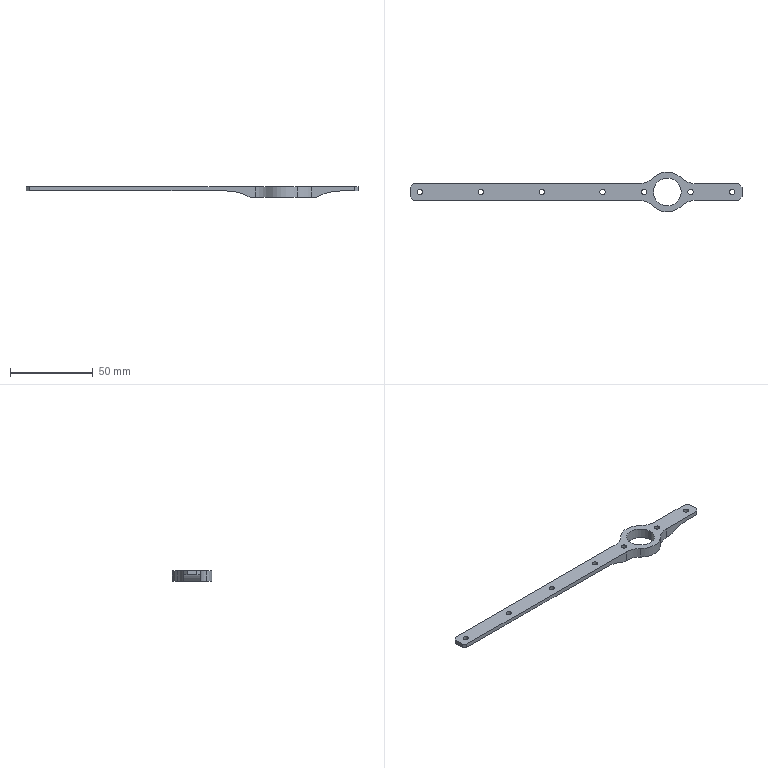Part | SolidWorks | features BaseBody 1 | 1 solid | 38 faces | box 200 x 24 x 6.35 mm | volume 6855 mm3 | cylinder 24 | plane 14 | commonest cylinder face diameters 3.2 x14 24 x6 16.667 x2 57.936 x2
STEP:
#1=CARTESIAN_POINT('',(46.666,0.,6.35));
#2=VERTEX_POINT('',#1);
#3=CARTESIAN_POINT('',(63.334,0.,6.35));
#4=VERTEX_POINT('',#3);
#5=CARTESIAN_POINT('',(55.,0.,6.35));
#6=DIRECTION('',(0.,0.,1.));
#7=DIRECTION('',(-1.,0.,0.));
#8=AXIS2_PLACEMENT_3D('',#5,#6,#7);
#9=CIRCLE('',#8,8.334);
#10=EDGE_CURVE('',#2,#4,#9,.T.);
#11=ORIENTED_EDGE('',*,*,#10,.T.);
#12=CARTESIAN_POINT('',(63.334,0.,0.));
#13=VERTEX_POINT('',#12);
#14=CARTESIAN_POINT('',(63.334,0.,6.35));
#15=DIRECTION('',(0.,0.,-1.));
#16=VECTOR('',#15,1000.);
#17=LINE('',#14,#16);
#18=EDGE_CURVE('',#4,#13,#17,.T.);
#19=ORIENTED_EDGE('',*,*,#18,.T.);
#20=CARTESIAN_POINT('',(46.666,0.,0.));
#21=VERTEX_POINT('',#20);
#22=CARTESIAN_POINT('',(55.,0.,0.));
#23=DIRECTION('',(0.,0.,-1.));
#24=DIRECTION('',(-1.,0.,0.));
#25=AXIS2_PLACEMENT_3D('',#22,#23,#24);
#26=CIRCLE('',#25,8.334);
#27=EDGE_CURVE('',#13,#21,#26,.T.);
#28=ORIENTED_EDGE('',*,*,#27,.T.);
#29=CARTESIAN_POINT('',(46.666,0.,6.35));
#30=DIRECTION('',(0.,0.,-1.));
#31=VECTOR('',#30,1000.);
#32=LINE('',#29,#31);
#33=EDGE_CURVE('',#2,#21,#32,.T.);
#34=ORIENTED_EDGE('',*,*,#33,.F.);
#35=EDGE_LOOP('',(#11,#19,#28,#34));
#36=FACE_OUTER_BOUND('',#35,.T.);
#37=CARTESIAN_POINT('',(55.,0.,6.35));
#38=DIRECTION('',(0.,0.,-1.));
#39=DIRECTION('',(-1.,0.,0.));
#40=AXIS2_PLACEMENT_3D('',#37,#38,#39);
#41=CYLINDRICAL_SURFACE('',#40,8.334);
#42=ADVANCED_FACE('',(#36),#41,.F.);
#43=CARTESIAN_POINT('',(67.4,0.,6.35));
#44=VERTEX_POINT('',#43);
#45=CARTESIAN_POINT('',(70.6,0.,6.35));
#46=VERTEX_POINT('',#45);
#47=CARTESIAN_POINT('',(69.,0.,6.35));
#48=DIRECTION('',(0.,0.,1.));
#49=DIRECTION('',(-1.,0.,0.));
#50=AXIS2_PLACEMENT_3D('',#47,#48,#49);
#51=CIRCLE('',#50,1.6);
#52=EDGE_CURVE('',#44,#46,#51,.T.);
#53=ORIENTED_EDGE('',*,*,#52,.T.);
#54=CARTESIAN_POINT('',(70.6,0.,0.));
#55=VERTEX_POINT('',#54);
#56=CARTESIAN_POINT('',(70.6,0.,6.35));
#57=DIRECTION('',(0.,0.,-1.));
#58=VECTOR('',#57,1000.);
#59=LINE('',#56,#58);
#60=EDGE_CURVE('',#46,#55,#59,.T.);
#61=ORIENTED_EDGE('',*,*,#60,.T.);
#62=CARTESIAN_POINT('',(67.4,0.,0.));
#63=VERTEX_POINT('',#62);
#64=CARTESIAN_POINT('',(69.,0.,0.));
#65=DIRECTION('',(0.,0.,1.));
#66=DIRECTION('',(-1.,0.,0.));
#67=AXIS2_PLACEMENT_3D('',#64,#65,#66);
#68=CIRCLE('',#67,1.6);
#69=EDGE_CURVE('',#63,#55,#68,.T.);
#70=ORIENTED_EDGE('',*,*,#69,.F.);
#71=CARTESIAN_POINT('',(67.4,0.,6.35));
#72=DIRECTION('',(0.,0.,-1.));
#73=VECTOR('',#72,1000.);
#74=LINE('',#71,#73);
#75=EDGE_CURVE('',#44,#63,#74,.T.);
#76=ORIENTED_EDGE('',*,*,#75,.F.);
#77=EDGE_LOOP('',(#53,#61,#70,#76));
#78=FACE_OUTER_BOUND('',#77,.T.);
#79=CARTESIAN_POINT('',(69.,0.,6.35));
#80=DIRECTION('',(0.,0.,-1.));
#81=DIRECTION('',(-1.,0.,0.));
#82=AXIS2_PLACEMENT_3D('',#79,#80,#81);
#83=CYLINDRICAL_SURFACE('',#82,1.6);
#84=ADVANCED_FACE('',(#78),#83,.F.);
#85=CARTESIAN_POINT('',(39.4,0.,6.35));
#86=VERTEX_POINT('',#85);
#87=CARTESIAN_POINT('',(42.6,0.,6.35));
#88=VERTEX_POINT('',#87);
#89=CARTESIAN_POINT('',(41.,0.,6.35));
#90=DIRECTION('',(0.,0.,1.));
#91=DIRECTION('',(-1.,0.,0.));
#92=AXIS2_PLACEMENT_3D('',#89,#90,#91);
#93=CIRCLE('',#92,1.6);
#94=EDGE_CURVE('',#86,#88,#93,.T.);
#95=ORIENTED_EDGE('',*,*,#94,.T.);
#96=CARTESIAN_POINT('',(42.6,0.,0.));
#97=VERTEX_POINT('',#96);
#98=CARTESIAN_POINT('',(42.6,0.,6.35));
#99=DIRECTION('',(0.,0.,-1.));
#100=VECTOR('',#99,1000.);
#101=LINE('',#98,#100);
#102=EDGE_CURVE('',#88,#97,#101,.T.);
#103=ORIENTED_EDGE('',*,*,#102,.T.);
#104=CARTESIAN_POINT('',(39.4,0.,0.));
#105=VERTEX_POINT('',#104);
#106=CARTESIAN_POINT('',(41.,0.,0.));
#107=DIRECTION('',(0.,0.,1.));
#108=DIRECTION('',(-1.,0.,0.));
#109=AXIS2_PLACEMENT_3D('',#106,#107,#108);
#110=CIRCLE('',#109,1.6);
#111=EDGE_CURVE('',#105,#97,#110,.T.);
#112=ORIENTED_EDGE('',*,*,#111,.F.);
#113=CARTESIAN_POINT('',(39.4,0.,6.35));
#114=DIRECTION('',(0.,0.,-1.));
#115=VECTOR('',#114,1000.);
#116=LINE('',#113,#115);
#117=EDGE_CURVE('',#86,#105,#116,.T.);
#118=ORIENTED_EDGE('',*,*,#117,.F.);
#119=EDGE_LOOP('',(#95,#103,#112,#118));
#120=FACE_OUTER_BOUND('',#119,.T.);
#121=CARTESIAN_POINT('',(41.,0.,6.35));
#122=DIRECTION('',(0.,0.,-1.));
#123=DIRECTION('',(-1.,0.,0.));
#124=AXIS2_PLACEMENT_3D('',#121,#122,#123);
#125=CYLINDRICAL_SURFACE('',#124,1.6);
#126=ADVANCED_FACE('',(#120),#125,.F.);
#127=CARTESIAN_POINT('',(-58.9,0.,6.35));
#128=VERTEX_POINT('',#127);
#129=CARTESIAN_POINT('',(-55.7,0.,6.35));
#130=VERTEX_POINT('',#129);
#131=CARTESIAN_POINT('',(-57.3,0.,6.35));
#132=DIRECTION('',(0.,0.,1.));
#133=DIRECTION('',(-1.,0.,0.));
#134=AXIS2_PLACEMENT_3D('',#131,#132,#133);
#135=CIRCLE('',#134,1.6);
#136=EDGE_CURVE('',#128,#130,#135,.T.);
#137=ORIENTED_EDGE('',*,*,#136,.T.);
#138=CARTESIAN_POINT('',(-55.7,0.,3.81));
#139=VERTEX_POINT('',#138);
#140=CARTESIAN_POINT('',(-55.7,0.,6.35));
#141=DIRECTION('',(0.,0.,-1.));
#142=VECTOR('',#141,1000.);
#143=LINE('',#140,#142);
#144=EDGE_CURVE('',#130,#139,#143,.T.);
#145=ORIENTED_EDGE('',*,*,#144,.T.);
#146=CARTESIAN_POINT('',(-58.9,0.,3.81));
#147=VERTEX_POINT('',#146);
#148=CARTESIAN_POINT('',(-57.3,0.,3.81));
#149=DIRECTION('',(0.,0.,-1.));
#150=DIRECTION('',(-1.,0.,0.));
#151=AXIS2_PLACEMENT_3D('',#148,#149,#150);
#152=CIRCLE('',#151,1.6);
#153=EDGE_CURVE('',#139,#147,#152,.T.);
#154=ORIENTED_EDGE('',*,*,#153,.T.);
#155=CARTESIAN_POINT('',(-58.9,0.,6.35));
#156=DIRECTION('',(0.,0.,-1.));
#157=VECTOR('',#156,1000.);
#158=LINE('',#155,#157);
#159=EDGE_CURVE('',#128,#147,#158,.T.);
#160=ORIENTED_EDGE('',*,*,#159,.F.);
#161=EDGE_LOOP('',(#137,#145,#154,#160));
#162=FACE_OUTER_BOUND('',#161,.T.);
#163=CARTESIAN_POINT('',(-57.3,0.,6.35));
#164=DIRECTION('',(0.,0.,-1.));
#165=DIRECTION('',(-1.,0.,0.));
#166=AXIS2_PLACEMENT_3D('',#163,#164,#165);
#167=CYLINDRICAL_SURFACE('',#166,1.6);
#168=ADVANCED_FACE('',(#162),#167,.F.);
#169=CARTESIAN_POINT('',(-22.25,0.,6.35));
#170=VERTEX_POINT('',#169);
#171=CARTESIAN_POINT('',(-19.05,0.,6.35));
#172=VERTEX_POINT('',#171);
#173=CARTESIAN_POINT('',(-20.65,0.,6.35));
#174=DIRECTION('',(0.,0.,1.));
#175=DIRECTION('',(-1.,0.,0.));
#176=AXIS2_PLACEMENT_3D('',#173,#174,#175);
#177=CIRCLE('',#176,1.6);
#178=EDGE_CURVE('',#170,#172,#177,.T.);
#179=ORIENTED_EDGE('',*,*,#178,.T.);
#180=CARTESIAN_POINT('',(-19.05,0.,3.81));
#181=VERTEX_POINT('',#180);
#182=CARTESIAN_POINT('',(-19.05,0.,6.35));
#183=DIRECTION('',(0.,0.,-1.));
#184=VECTOR('',#183,1000.);
#185=LINE('',#182,#184);
#186=EDGE_CURVE('',#172,#181,#185,.T.);
#187=ORIENTED_EDGE('',*,*,#186,.T.);
#188=CARTESIAN_POINT('',(-22.25,0.,3.81));
#189=VERTEX_POINT('',#188);
#190=CARTESIAN_POINT('',(-20.65,0.,3.81));
#191=DIRECTION('',(0.,0.,-1.));
#192=DIRECTION('',(-1.,0.,0.));
#193=AXIS2_PLACEMENT_3D('',#190,#191,#192);
#194=CIRCLE('',#193,1.6);
#195=EDGE_CURVE('',#181,#189,#194,.T.);
#196=ORIENTED_EDGE('',*,*,#195,.T.);
#197=CARTESIAN_POINT('',(-22.25,0.,6.35));
#198=DIRECTION('',(0.,0.,-1.));
#199=VECTOR('',#198,1000.);
#200=LINE('',#197,#199);
#201=EDGE_CURVE('',#170,#189,#200,.T.);
#202=ORIENTED_EDGE('',*,*,#201,.F.);
#203=EDGE_LOOP('',(#179,#187,#196,#202));
#204=FACE_OUTER_BOUND('',#203,.T.);
#205=CARTESIAN_POINT('',(-20.65,0.,6.35));
#206=DIRECTION('',(0.,0.,-1.));
#207=DIRECTION('',(-1.,0.,0.));
#208=AXIS2_PLACEMENT_3D('',#205,#206,#207);
#209=CYLINDRICAL_SURFACE('',#208,1.6);
#210=ADVANCED_FACE('',(#204),#209,.F.);
#211=CARTESIAN_POINT('',(14.4,0.,6.35));
#212=VERTEX_POINT('',#211);
#213=CARTESIAN_POINT('',(17.6,0.,6.35));
#214=VERTEX_POINT('',#213);
#215=CARTESIAN_POINT('',(16.,0.,6.35));
#216=DIRECTION('',(0.,0.,1.));
#217=DIRECTION('',(-1.,0.,0.));
#218=AXIS2_PLACEMENT_3D('',#215,#216,#217);
#219=CIRCLE('',#218,1.6);
#220=EDGE_CURVE('',#212,#214,#219,.T.);
#221=ORIENTED_EDGE('',*,*,#220,.T.);
#222=CARTESIAN_POINT('',(17.6,0.,3.81));
#223=VERTEX_POINT('',#222);
#224=CARTESIAN_POINT('',(17.6,0.,6.35));
#225=DIRECTION('',(0.,0.,-1.));
#226=VECTOR('',#225,1000.);
#227=LINE('',#224,#226);
#228=EDGE_CURVE('',#214,#223,#227,.T.);
#229=ORIENTED_EDGE('',*,*,#228,.T.);
#230=CARTESIAN_POINT('',(14.4,0.,3.81));
#231=VERTEX_POINT('',#230);
#232=CARTESIAN_POINT('',(16.,0.,3.81));
#233=DIRECTION('',(0.,0.,-1.));
#234=DIRECTION('',(-1.,0.,0.));
#235=AXIS2_PLACEMENT_3D('',#232,#233,#234);
#236=CIRCLE('',#235,1.6);
#237=EDGE_CURVE('',#223,#231,#236,.T.);
#238=ORIENTED_EDGE('',*,*,#237,.T.);
#239=CARTESIAN_POINT('',(14.4,0.,6.35));
#240=DIRECTION('',(0.,0.,-1.));
#241=VECTOR('',#240,1000.);
#242=LINE('',#239,#241);
#243=EDGE_CURVE('',#212,#231,#242,.T.);
#244=ORIENTED_EDGE('',*,*,#243,.F.);
#245=EDGE_LOOP('',(#221,#229,#238,#244));
#246=FACE_OUTER_BOUND('',#245,.T.);
#247=CARTESIAN_POINT('',(16.,0.,6.35));
#248=DIRECTION('',(0.,0.,-1.));
#249=DIRECTION('',(-1.,0.,0.));
#250=AXIS2_PLACEMENT_3D('',#247,#248,#249);
#251=CYLINDRICAL_SURFACE('',#250,1.6);
#252=ADVANCED_FACE('',(#246),#251,.F.);
#253=CARTESIAN_POINT('',(-95.6,0.,6.35));
#254=VERTEX_POINT('',#253);
#255=CARTESIAN_POINT('',(-92.4,0.,6.35));
#256=VERTEX_POINT('',#255);
#257=CARTESIAN_POINT('',(-94.,0.,6.35));
#258=DIRECTION('',(0.,0.,1.));
#259=DIRECTION('',(-1.,0.,0.));
#260=AXIS2_PLACEMENT_3D('',#257,#258,#259);
#261=CIRCLE('',#260,1.6);
#262=EDGE_CURVE('',#254,#256,#261,.T.);
#263=ORIENTED_EDGE('',*,*,#262,.T.);
#264=CARTESIAN_POINT('',(-92.4,0.,3.81));
#265=VERTEX_POINT('',#264);
#266=CARTESIAN_POINT('',(-92.4,0.,6.35));
#267=DIRECTION('',(0.,0.,-1.));
#268=VECTOR('',#267,1000.);
#269=LINE('',#266,#268);
#270=EDGE_CURVE('',#256,#265,#269,.T.);
#271=ORIENTED_EDGE('',*,*,#270,.T.);
#272=CARTESIAN_POINT('',(-95.6,0.,3.81));
#273=VERTEX_POINT('',#272);
#274=CARTESIAN_POINT('',(-94.,0.,3.81));
#275=DIRECTION('',(0.,0.,-1.));
#276=DIRECTION('',(-1.,0.,0.));
#277=AXIS2_PLACEMENT_3D('',#274,#275,#276);
#278=CIRCLE('',#277,1.6);
#279=EDGE_CURVE('',#265,#273,#278,.T.);
#280=ORIENTED_EDGE('',*,*,#279,.T.);
#281=CARTESIAN_POINT('',(-95.6,0.,6.35));
#282=DIRECTION('',(0.,0.,-1.));
#283=VECTOR('',#282,1000.);
#284=LINE('',#281,#283);
#285=EDGE_CURVE('',#254,#273,#284,.T.);
#286=ORIENTED_EDGE('',*,*,#285,.F.);
#287=EDGE_LOOP('',(#263,#271,#280,#286));
#288=FACE_OUTER_BOUND('',#287,.T.);
#289=CARTESIAN_POINT('',(-94.,0.,6.35));
#290=DIRECTION('',(0.,0.,-1.));
#291=DIRECTION('',(-1.,0.,0.));
#292=AXIS2_PLACEMENT_3D('',#289,#290,#291);
#293=CYLINDRICAL_SURFACE('',#292,1.6);
#294=ADVANCED_FACE('',(#288),#293,.F.);
#295=CARTESIAN_POINT('',(92.4,0.,6.35));
#296=VERTEX_POINT('',#295);
#297=CARTESIAN_POINT('',(95.6,0.,6.35));
#298=VERTEX_POINT('',#297);
#299=CARTESIAN_POINT('',(94.,0.,6.35));
#300=DIRECTION('',(0.,0.,1.));
#301=DIRECTION('',(-1.,0.,0.));
#302=AXIS2_PLACEMENT_3D('',#299,#300,#301);
#303=CIRCLE('',#302,1.6);
#304=EDGE_CURVE('',#296,#298,#303,.T.);
#305=ORIENTED_EDGE('',*,*,#304,.T.);
#306=CARTESIAN_POINT('',(95.6,0.,3.81));
#307=VERTEX_POINT('',#306);
#308=CARTESIAN_POINT('',(95.6,0.,6.35));
#309=DIRECTION('',(0.,0.,-1.));
#310=VECTOR('',#309,1000.);
#311=LINE('',#308,#310);
#312=EDGE_CURVE('',#298,#307,#311,.T.);
#313=ORIENTED_EDGE('',*,*,#312,.T.);
#314=CARTESIAN_POINT('',(92.4,0.,3.81));
#315=VERTEX_POINT('',#314);
#316=CARTESIAN_POINT('',(94.,0.,3.81));
#317=DIRECTION('',(0.,0.,-1.));
#318=DIRECTION('',(-1.,0.,0.));
#319=AXIS2_PLACEMENT_3D('',#316,#317,#318);
#320=CIRCLE('',#319,1.6);
#321=EDGE_CURVE('',#307,#315,#320,.T.);
#322=ORIENTED_EDGE('',*,*,#321,.T.);
#323=CARTESIAN_POINT('',(92.4,0.,6.35));
#324=DIRECTION('',(0.,0.,-1.));
#325=VECTOR('',#324,1000.);
#326=LINE('',#323,#325);
#327=EDGE_CURVE('',#296,#315,#326,.T.);
#328=ORIENTED_EDGE('',*,*,#327,.F.);
#329=EDGE_LOOP('',(#305,#313,#322,#328));
#330=FACE_OUTER_BOUND('',#329,.T.);
#331=CARTESIAN_POINT('',(94.,0.,6.35));
#332=DIRECTION('',(0.,0.,-1.));
#333=DIRECTION('',(-1.,0.,0.));
#334=AXIS2_PLACEMENT_3D('',#331,#332,#333);
#335=CYLINDRICAL_SURFACE('',#334,1.6);
#336=ADVANCED_FACE('',(#330),#335,.F.);
#337=ORIENTED_EDGE('',*,*,#18,.F.);
#338=CARTESIAN_POINT('',(55.,0.,6.35));
#339=DIRECTION('',(0.,0.,1.));
#340=DIRECTION('',(-1.,0.,0.));
#341=AXIS2_PLACEMENT_3D('',#338,#339,#340);
#342=CIRCLE('',#341,8.334);
#343=EDGE_CURVE('',#4,#2,#342,.T.);
#344=ORIENTED_EDGE('',*,*,#343,.T.);
#345=ORIENTED_EDGE('',*,*,#33,.T.);
#346=CARTESIAN_POINT('',(55.,0.,0.));
#347=DIRECTION('',(0.,0.,-1.));
#348=DIRECTION('',(-1.,0.,0.));
#349=AXIS2_PLACEMENT_3D('',#346,#347,#348);
#350=CIRCLE('',#349,8.334);
#351=EDGE_CURVE('',#21,#13,#350,.T.);
#352=ORIENTED_EDGE('',*,*,#351,.T.);
#353=EDGE_LOOP('',(#337,#344,#345,#352));
#354=FACE_OUTER_BOUND('',#353,.T.);
#355=CARTESIAN_POINT('',(55.,0.,6.35));
#356=DIRECTION('',(0.,0.,-1.));
#357=DIRECTION('',(-1.,0.,0.));
#358=AXIS2_PLACEMENT_3D('',#355,#356,#357);
#359=CYLINDRICAL_SURFACE('',#358,8.334);
#360=ADVANCED_FACE('',(#354),#359,.F.);
#361=ORIENTED_EDGE('',*,*,#351,.F.);
#362=ORIENTED_EDGE('',*,*,#27,.F.);
#363=EDGE_LOOP('',(#361,#362));
#364=FACE_BOUND('',#363,.T.);
#365=ORIENTED_EDGE('',*,*,#69,.T.);
#366=CARTESIAN_POINT('',(69.,0.,0.));
#367=DIRECTION('',(0.,0.,1.));
#368=DIRECTION('',(-1.,0.,0.));
#369=AXIS2_PLACEMENT_3D('',#366,#367,#368);
#370=CIRCLE('',#369,1.6);
#371=EDGE_CURVE('',#55,#63,#370,.T.);
#372=ORIENTED_EDGE('',*,*,#371,.T.);
#373=EDGE_LOOP('',(#365,#372));
#374=FACE_BOUND('',#373,.T.);
#375=ORIENTED_EDGE('',*,*,#111,.T.);
#376=CARTESIAN_POINT('',(41.,0.,0.));
#377=DIRECTION('',(0.,0.,1.));
#378=DIRECTION('',(-1.,0.,0.));
#379=AXIS2_PLACEMENT_3D('',#376,#377,#378);
#380=CIRCLE('',#379,1.6);
#381=EDGE_CURVE('',#97,#105,#380,.T.);
#382=ORIENTED_EDGE('',*,*,#381,.T.);
#383=EDGE_LOOP('',(#375,#382));
#384=FACE_BOUND('',#383,.T.);
#385=CARTESIAN_POINT('',(63.471,8.5,0.));
#386=VERTEX_POINT('',#385);
#387=CARTESIAN_POINT('',(71.941,5.,0.));
#388=VERTEX_POINT('',#387);
#389=CARTESIAN_POINT('',(71.941,17.,0.));
#390=DIRECTION('',(0.,0.,1.));
#391=DIRECTION('',(-1.,0.,0.));
#392=AXIS2_PLACEMENT_3D('',#389,#390,#391);
#393=CIRCLE('',#392,12.);
#394=EDGE_CURVE('',#386,#388,#393,.T.);
#395=ORIENTED_EDGE('',*,*,#394,.T.);
#396=CARTESIAN_POINT('',(75.,5.,0.));
#397=VERTEX_POINT('',#396);
#398=CARTESIAN_POINT('',(55.,5.,0.));
#399=DIRECTION('',(1.,0.,0.));
#400=VECTOR('',#399,1000.);
#401=LINE('',#398,#400);
#402=EDGE_CURVE('',#388,#397,#401,.T.);
#403=ORIENTED_EDGE('',*,*,#402,.T.);
#404=CARTESIAN_POINT('',(75.,-5.,0.));
#405=VERTEX_POINT('',#404);
#406=CARTESIAN_POINT('',(75.,0.,0.));
#407=DIRECTION('',(0.,-1.,0.));
#408=VECTOR('',#407,1000.);
#409=LINE('',#406,#408);
#410=EDGE_CURVE('',#397,#405,#409,.T.);
#411=ORIENTED_EDGE('',*,*,#410,.T.);
#412=CARTESIAN_POINT('',(71.941,-5.,0.));
#413=VERTEX_POINT('',#412);
#414=CARTESIAN_POINT('',(55.,-5.,0.));
#415=DIRECTION('',(-1.,0.,0.));
#416=VECTOR('',#415,1000.);
#417=LINE('',#414,#416);
#418=EDGE_CURVE('',#405,#413,#417,.T.);
#419=ORIENTED_EDGE('',*,*,#418,.T.);
#420=CARTESIAN_POINT('',(63.471,-8.5,0.));
#421=VERTEX_POINT('',#420);
#422=CARTESIAN_POINT('',(71.941,-17.,0.));
#423=DIRECTION('',(0.,0.,1.));
#424=DIRECTION('',(-1.,0.,0.));
#425=AXIS2_PLACEMENT_3D('',#422,#423,#424);
#426=CIRCLE('',#425,12.);
#427=EDGE_CURVE('',#413,#421,#426,.T.);
#428=ORIENTED_EDGE('',*,*,#427,.T.);
#429=CARTESIAN_POINT('',(46.529,-8.5,0.));
#430=VERTEX_POINT('',#429);
#431=CARTESIAN_POINT('',(55.,0.,0.));
#432=DIRECTION('',(0.,0.,-1.));
#433=DIRECTION('',(-1.,0.,0.));
#434=AXIS2_PLACEMENT_3D('',#431,#432,#433);
#435=CIRCLE('',#434,12.);
#436=EDGE_CURVE('',#421,#430,#435,.T.);
#437=ORIENTED_EDGE('',*,*,#436,.T.);
#438=CARTESIAN_POINT('',(38.059,-5.,0.));
#439=VERTEX_POINT('',#438);
#440=CARTESIAN_POINT('',(38.059,-17.,0.));
#441=DIRECTION('',(0.,0.,1.));
#442=DIRECTION('',(-1.,0.,0.));
#443=AXIS2_PLACEMENT_3D('',#440,#441,#442);
#444=CIRCLE('',#443,12.);
#445=EDGE_CURVE('',#430,#439,#444,.T.);
#446=ORIENTED_EDGE('',*,*,#445,.T.);
#447=CARTESIAN_POINT('',(35.,-5.,0.));
#448=VERTEX_POINT('',#447);
#449=CARTESIAN_POINT('',(55.,-5.,0.));
#450=DIRECTION('',(-1.,0.,0.));
#451=VECTOR('',#450,1000.);
#452=LINE('',#449,#451);
#453=EDGE_CURVE('',#439,#448,#452,.T.);
#454=ORIENTED_EDGE('',*,*,#453,.T.);
#455=CARTESIAN_POINT('',(35.,5.,0.));
#456=VERTEX_POINT('',#455);
#457=CARTESIAN_POINT('',(35.,0.,0.));
#458=DIRECTION('',(0.,1.,0.));
#459=VECTOR('',#458,1000.);
#460=LINE('',#457,#459);
#461=EDGE_CURVE('',#448,#456,#460,.T.);
#462=ORIENTED_EDGE('',*,*,#461,.T.);
#463=CARTESIAN_POINT('',(38.059,5.,0.));
#464=VERTEX_POINT('',#463);
#465=CARTESIAN_POINT('',(55.,5.,0.));
#466=DIRECTION('',(1.,0.,0.));
#467=VECTOR('',#466,1000.);
#468=LINE('',#465,#467);
#469=EDGE_CURVE('',#456,#464,#468,.T.);
#470=ORIENTED_EDGE('',*,*,#469,.T.);
#471=CARTESIAN_POINT('',(46.529,8.5,0.));
#472=VERTEX_POINT('',#471);
#473=CARTESIAN_POINT('',(38.059,17.,0.));
#474=DIRECTION('',(0.,0.,1.));
#475=DIRECTION('',(-1.,0.,0.));
#476=AXIS2_PLACEMENT_3D('',#473,#474,#475);
#477=CIRCLE('',#476,12.);
#478=EDGE_CURVE('',#464,#472,#477,.T.);
#479=ORIENTED_EDGE('',*,*,#478,.T.);
#480=CARTESIAN_POINT('',(55.,0.,0.));
#481=DIRECTION('',(0.,0.,-1.));
#482=DIRECTION('',(-1.,0.,0.));
#483=AXIS2_PLACEMENT_3D('',#480,#481,#482);
#484=CIRCLE('',#483,12.);
#485=EDGE_CURVE('',#472,#386,#484,.T.);
#486=ORIENTED_EDGE('',*,*,#485,.T.);
#487=EDGE_LOOP('',(#395,#403,#411,#419,#428,#437,#446,#454,#462,#470,#479,#486));
#488=FACE_OUTER_BOUND('',#487,.T.);
#489=CARTESIAN_POINT('',(75.,-12.144,0.));
#490=DIRECTION('',(0.,0.,-1.));
#491=DIRECTION('',(-1.,0.,0.));
#492=AXIS2_PLACEMENT_3D('',#489,#490,#491);
#493=PLANE('',#492);
#494=ADVANCED_FACE('',(#364,#374,#384,#488),#493,.T.);
#495=ORIENTED_EDGE('',*,*,#10,.F.);
#496=ORIENTED_EDGE('',*,*,#343,.F.);
#497=EDGE_LOOP('',(#495,#496));
#498=FACE_BOUND('',#497,.T.);
#499=ORIENTED_EDGE('',*,*,#136,.F.);
#500=CARTESIAN_POINT('',(-57.3,0.,6.35));
#501=DIRECTION('',(0.,0.,1.));
#502=DIRECTION('',(-1.,0.,0.));
#503=AXIS2_PLACEMENT_3D('',#500,#501,#502);
#504=CIRCLE('',#503,1.6);
#505=EDGE_CURVE('',#130,#128,#504,.T.);
#506=ORIENTED_EDGE('',*,*,#505,.F.);
#507=EDGE_LOOP('',(#499,#506));
#508=FACE_BOUND('',#507,.T.);
#509=ORIENTED_EDGE('',*,*,#178,.F.);
#510=CARTESIAN_POINT('',(-20.65,0.,6.35));
#511=DIRECTION('',(0.,0.,1.));
#512=DIRECTION('',(-1.,0.,0.));
#513=AXIS2_PLACEMENT_3D('',#510,#511,#512);
#514=CIRCLE('',#513,1.6);
#515=EDGE_CURVE('',#172,#170,#514,.T.);
#516=ORIENTED_EDGE('',*,*,#515,.F.);
#517=EDGE_LOOP('',(#509,#516));
#518=FACE_BOUND('',#517,.T.);
#519=ORIENTED_EDGE('',*,*,#220,.F.);
#520=CARTESIAN_POINT('',(16.,0.,6.35));
#521=DIRECTION('',(0.,0.,1.));
#522=DIRECTION('',(-1.,0.,0.));
#523=AXIS2_PLACEMENT_3D('',#520,#521,#522);
#524=CIRCLE('',#523,1.6);
#525=EDGE_CURVE('',#214,#212,#524,.T.);
#526=ORIENTED_EDGE('',*,*,#525,.F.);
#527=EDGE_LOOP('',(#519,#526));
#528=FACE_BOUND('',#527,.T.);
#529=ORIENTED_EDGE('',*,*,#262,.F.);
#530=CARTESIAN_POINT('',(-94.,0.,6.35));
#531=DIRECTION('',(0.,0.,1.));
#532=DIRECTION('',(-1.,0.,0.));
#533=AXIS2_PLACEMENT_3D('',#530,#531,#532);
#534=CIRCLE('',#533,1.6);
#535=EDGE_CURVE('',#256,#254,#534,.T.);
#536=ORIENTED_EDGE('',*,*,#535,.F.);
#537=EDGE_LOOP('',(#529,#536));
#538=FACE_BOUND('',#537,.T.);
#539=ORIENTED_EDGE('',*,*,#94,.F.);
#540=CARTESIAN_POINT('',(41.,0.,6.35));
#541=DIRECTION('',(0.,0.,1.));
#542=DIRECTION('',(-1.,0.,0.));
#543=AXIS2_PLACEMENT_3D('',#540,#541,#542);
#544=CIRCLE('',#543,1.6);
#545=EDGE_CURVE('',#88,#86,#544,.T.);
#546=ORIENTED_EDGE('',*,*,#545,.F.);
#547=EDGE_LOOP('',(#539,#546));
#548=FACE_BOUND('',#547,.T.);
#549=ORIENTED_EDGE('',*,*,#304,.F.);
#550=CARTESIAN_POINT('',(94.,0.,6.35));
#551=DIRECTION('',(0.,0.,1.));
#552=DIRECTION('',(-1.,0.,0.));
#553=AXIS2_PLACEMENT_3D('',#550,#551,#552);
#554=CIRCLE('',#553,1.6);
#555=EDGE_CURVE('',#298,#296,#554,.T.);
#556=ORIENTED_EDGE('',*,*,#555,.F.);
#557=EDGE_LOOP('',(#549,#556));
#558=FACE_BOUND('',#557,.T.);
#559=ORIENTED_EDGE('',*,*,#52,.F.);
#560=CARTESIAN_POINT('',(69.,0.,6.35));
#561=DIRECTION('',(0.,0.,1.));
#562=DIRECTION('',(-1.,0.,0.));
#563=AXIS2_PLACEMENT_3D('',#560,#561,#562);
#564=CIRCLE('',#563,1.6);
#565=EDGE_CURVE('',#46,#44,#564,.T.);
#566=ORIENTED_EDGE('',*,*,#565,.F.);
#567=EDGE_LOOP('',(#559,#566));
#568=FACE_BOUND('',#567,.T.);
#569=CARTESIAN_POINT('',(98.,-5.,6.35));
#570=VERTEX_POINT('',#569);
#571=CARTESIAN_POINT('',(71.941,-5.,6.35));
#572=VERTEX_POINT('',#571);
#573=CARTESIAN_POINT('',(0.,-5.,6.35));
#574=DIRECTION('',(-1.,0.,0.));
#575=VECTOR('',#574,1000.);
#576=LINE('',#573,#575);
#577=EDGE_CURVE('',#570,#572,#576,.T.);
#578=ORIENTED_EDGE('',*,*,#577,.F.);
#579=CARTESIAN_POINT('',(100.,-3.,6.35));
#580=VERTEX_POINT('',#579);
#581=CARTESIAN_POINT('',(100.,-3.,6.35));
#582=DIRECTION('',(-0.7071,-0.7071,0.));
#583=VECTOR('',#582,1000.);
#584=LINE('',#581,#583);
#585=EDGE_CURVE('',#580,#570,#584,.T.);
#586=ORIENTED_EDGE('',*,*,#585,.F.);
#587=CARTESIAN_POINT('',(100.,3.,6.35));
#588=VERTEX_POINT('',#587);
#589=CARTESIAN_POINT('',(100.,0.,6.35));
#590=DIRECTION('',(0.,-1.,0.));
#591=VECTOR('',#590,1000.);
#592=LINE('',#589,#591);
#593=EDGE_CURVE('',#588,#580,#592,.T.);
#594=ORIENTED_EDGE('',*,*,#593,.F.);
#595=CARTESIAN_POINT('',(98.,5.,6.35));
#596=VERTEX_POINT('',#595);
#597=CARTESIAN_POINT('',(98.,5.,6.35));
#598=DIRECTION('',(0.7071,-0.7071,0.));
#599=VECTOR('',#598,1000.);
#600=LINE('',#597,#599);
#601=EDGE_CURVE('',#596,#588,#600,.T.);
#602=ORIENTED_EDGE('',*,*,#601,.F.);
#603=CARTESIAN_POINT('',(71.941,5.,6.35));
#604=VERTEX_POINT('',#603);
#605=CARTESIAN_POINT('',(0.,5.,6.35));
#606=DIRECTION('',(1.,0.,0.));
#607=VECTOR('',#606,1000.);
#608=LINE('',#605,#607);
#609=EDGE_CURVE('',#604,#596,#608,.T.);
#610=ORIENTED_EDGE('',*,*,#609,.F.);
#611=CARTESIAN_POINT('',(63.471,8.5,6.35));
#612=VERTEX_POINT('',#611);
#613=CARTESIAN_POINT('',(71.941,17.,6.35));
#614=DIRECTION('',(0.,0.,1.));
#615=DIRECTION('',(-1.,0.,0.));
#616=AXIS2_PLACEMENT_3D('',#613,#614,#615);
#617=CIRCLE('',#616,12.);
#618=EDGE_CURVE('',#612,#604,#617,.T.);
#619=ORIENTED_EDGE('',*,*,#618,.F.);
#620=CARTESIAN_POINT('',(46.529,8.5,6.35));
#621=VERTEX_POINT('',#620);
#622=CARTESIAN_POINT('',(55.,0.,6.35));
#623=DIRECTION('',(0.,0.,-1.));
#624=DIRECTION('',(-1.,0.,0.));
#625=AXIS2_PLACEMENT_3D('',#622,#623,#624);
#626=CIRCLE('',#625,12.);
#627=EDGE_CURVE('',#621,#612,#626,.T.);
#628=ORIENTED_EDGE('',*,*,#627,.F.);
#629=CARTESIAN_POINT('',(38.059,5.,6.35));
#630=VERTEX_POINT('',#629);
#631=CARTESIAN_POINT('',(38.059,17.,6.35));
#632=DIRECTION('',(0.,0.,1.));
#633=DIRECTION('',(-1.,0.,0.));
#634=AXIS2_PLACEMENT_3D('',#631,#632,#633);
#635=CIRCLE('',#634,12.);
#636=EDGE_CURVE('',#630,#621,#635,.T.);
#637=ORIENTED_EDGE('',*,*,#636,.F.);
#638=CARTESIAN_POINT('',(-98.,5.,6.35));
#639=VERTEX_POINT('',#638);
#640=CARTESIAN_POINT('',(0.,5.,6.35));
#641=DIRECTION('',(1.,0.,0.));
#642=VECTOR('',#641,1000.);
#643=LINE('',#640,#642);
#644=EDGE_CURVE('',#639,#630,#643,.T.);
#645=ORIENTED_EDGE('',*,*,#644,.F.);
#646=CARTESIAN_POINT('',(-100.,3.,6.35));
#647=VERTEX_POINT('',#646);
#648=CARTESIAN_POINT('',(-100.,3.,6.35));
#649=DIRECTION('',(0.7071,0.7071,0.));
#650=VECTOR('',#649,1000.);
#651=LINE('',#648,#650);
#652=EDGE_CURVE('',#647,#639,#651,.T.);
#653=ORIENTED_EDGE('',*,*,#652,.F.);
#654=CARTESIAN_POINT('',(-100.,-3.,6.35));
#655=VERTEX_POINT('',#654);
#656=CARTESIAN_POINT('',(-100.,0.,6.35));
#657=DIRECTION('',(0.,1.,0.));
#658=VECTOR('',#657,1000.);
#659=LINE('',#656,#658);
#660=EDGE_CURVE('',#655,#647,#659,.T.);
#661=ORIENTED_EDGE('',*,*,#660,.F.);
#662=CARTESIAN_POINT('',(-98.,-5.,6.35));
#663=VERTEX_POINT('',#662);
#664=CARTESIAN_POINT('',(-98.,-5.,6.35));
#665=DIRECTION('',(-0.7071,0.7071,0.));
#666=VECTOR('',#665,1000.);
#667=LINE('',#664,#666);
#668=EDGE_CURVE('',#663,#655,#667,.T.);
#669=ORIENTED_EDGE('',*,*,#668,.F.);
#670=CARTESIAN_POINT('',(38.059,-5.,6.35));
#671=VERTEX_POINT('',#670);
#672=CARTESIAN_POINT('',(0.,-5.,6.35));
#673=DIRECTION('',(-1.,0.,0.));
#674=VECTOR('',#673,1000.);
#675=LINE('',#672,#674);
#676=EDGE_CURVE('',#671,#663,#675,.T.);
#677=ORIENTED_EDGE('',*,*,#676,.F.);
#678=CARTESIAN_POINT('',(46.529,-8.5,6.35));
#679=VERTEX_POINT('',#678);
#680=CARTESIAN_POINT('',(38.059,-17.,6.35));
#681=DIRECTION('',(0.,0.,1.));
#682=DIRECTION('',(-1.,0.,0.));
#683=AXIS2_PLACEMENT_3D('',#680,#681,#682);
#684=CIRCLE('',#683,12.);
#685=EDGE_CURVE('',#679,#671,#684,.T.);
#686=ORIENTED_EDGE('',*,*,#685,.F.);
#687=CARTESIAN_POINT('',(63.471,-8.5,6.35));
#688=VERTEX_POINT('',#687);
#689=CARTESIAN_POINT('',(55.,0.,6.35));
#690=DIRECTION('',(0.,0.,-1.));
#691=DIRECTION('',(-1.,0.,0.));
#692=AXIS2_PLACEMENT_3D('',#689,#690,#691);
#693=CIRCLE('',#692,12.);
#694=EDGE_CURVE('',#688,#679,#693,.T.);
#695=ORIENTED_EDGE('',*,*,#694,.F.);
#696=CARTESIAN_POINT('',(71.941,-17.,6.35));
#697=DIRECTION('',(0.,0.,1.));
#698=DIRECTION('',(-1.,0.,0.));
#699=AXIS2_PLACEMENT_3D('',#696,#697,#698);
#700=CIRCLE('',#699,12.);
#701=EDGE_CURVE('',#572,#688,#700,.T.);
#702=ORIENTED_EDGE('',*,*,#701,.F.);
#703=EDGE_LOOP('',(#578,#586,#594,#602,#610,#619,#628,#637,#645,#653,#661,#669,#677,#686,#695,#702));
#704=FACE_OUTER_BOUND('',#703,.T.);
#705=CARTESIAN_POINT('',(100.,-12.144,6.35));
#706=DIRECTION('',(0.,0.,-1.));
#707=DIRECTION('',(-1.,0.,0.));
#708=AXIS2_PLACEMENT_3D('',#705,#706,#707);
#709=PLANE('',#708);
#710=ADVANCED_FACE('',(#498,#508,#518,#528,#538,#548,#558,#568,#704),#709,.F.);
#711=ORIENTED_EDGE('',*,*,#60,.F.);
#712=ORIENTED_EDGE('',*,*,#565,.T.);
#713=ORIENTED_EDGE('',*,*,#75,.T.);
#714=ORIENTED_EDGE('',*,*,#371,.F.);
#715=EDGE_LOOP('',(#711,#712,#713,#714));
#716=FACE_OUTER_BOUND('',#715,.T.);
#717=CARTESIAN_POINT('',(69.,0.,6.35));
#718=DIRECTION('',(0.,0.,-1.));
#719=DIRECTION('',(-1.,0.,0.));
#720=AXIS2_PLACEMENT_3D('',#717,#718,#719);
#721=CYLINDRICAL_SURFACE('',#720,1.6);
#722=ADVANCED_FACE('',(#716),#721,.F.);
#723=ORIENTED_EDGE('',*,*,#102,.F.);
#724=ORIENTED_EDGE('',*,*,#545,.T.);
#725=ORIENTED_EDGE('',*,*,#117,.T.);
#726=ORIENTED_EDGE('',*,*,#381,.F.);
#727=EDGE_LOOP('',(#723,#724,#725,#726));
#728=FACE_OUTER_BOUND('',#727,.T.);
#729=CARTESIAN_POINT('',(41.,0.,6.35));
#730=DIRECTION('',(0.,0.,-1.));
#731=DIRECTION('',(-1.,0.,0.));
#732=AXIS2_PLACEMENT_3D('',#729,#730,#731);
#733=CYLINDRICAL_SURFACE('',#732,1.6);
#734=ADVANCED_FACE('',(#728),#733,.F.);
#735=CARTESIAN_POINT('',(89.36,5.,3.81));
#736=VERTEX_POINT('',#735);
#737=CARTESIAN_POINT('',(98.,5.,3.81));
#738=VERTEX_POINT('',#737);
#739=CARTESIAN_POINT('',(84.971,5.,3.81));
#740=DIRECTION('',(1.,0.,0.));
#741=VECTOR('',#740,1000.);
#742=LINE('',#739,#741);
#743=EDGE_CURVE('',#736,#738,#742,.T.);
#744=ORIENTED_EDGE('',*,*,#743,.F.);
#745=CARTESIAN_POINT('',(89.36,5.,-25.158));
#746=DIRECTION('',(0.,1.,0.));
#747=DIRECTION('',(-1.,0.,0.));
#748=AXIS2_PLACEMENT_3D('',#745,#746,#747);
#749=CIRCLE('',#748,28.968);
#750=EDGE_CURVE('',#397,#736,#749,.T.);
#751=ORIENTED_EDGE('',*,*,#750,.F.);
#752=ORIENTED_EDGE('',*,*,#402,.F.);
#753=CARTESIAN_POINT('',(71.941,5.,3.175));
#754=DIRECTION('',(0.,0.,-1.));
#755=VECTOR('',#754,1000.);
#756=LINE('',#753,#755);
#757=EDGE_CURVE('',#604,#388,#756,.T.);
#758=ORIENTED_EDGE('',*,*,#757,.F.);
#759=ORIENTED_EDGE('',*,*,#609,.T.);
#760=CARTESIAN_POINT('',(98.,5.,3.175));
#761=DIRECTION('',(0.,0.,1.));
#762=VECTOR('',#761,1000.);
#763=LINE('',#760,#762);
#764=EDGE_CURVE('',#738,#596,#763,.T.);
#765=ORIENTED_EDGE('',*,*,#764,.F.);
#766=EDGE_LOOP('',(#744,#751,#752,#758,#759,#765));
#767=FACE_OUTER_BOUND('',#766,.T.);
#768=CARTESIAN_POINT('',(71.941,5.,0.));
#769=DIRECTION('',(0.,-1.,0.));
#770=DIRECTION('',(1.,0.,0.));
#771=AXIS2_PLACEMENT_3D('',#768,#769,#770);
#772=PLANE('',#771);
#773=ADVANCED_FACE('',(#767),#772,.F.);
#774=ORIENTED_EDGE('',*,*,#618,.T.);
#775=ORIENTED_EDGE('',*,*,#757,.T.);
#776=ORIENTED_EDGE('',*,*,#394,.F.);
#777=CARTESIAN_POINT('',(63.471,8.5,3.175));
#778=DIRECTION('',(0.,0.,1.));
#779=VECTOR('',#778,1000.);
#780=LINE('',#777,#779);
#781=EDGE_CURVE('',#386,#612,#780,.T.);
#782=ORIENTED_EDGE('',*,*,#781,.T.);
#783=EDGE_LOOP('',(#774,#775,#776,#782));
#784=FACE_OUTER_BOUND('',#783,.T.);
#785=CARTESIAN_POINT('',(71.941,17.,6.35));
#786=DIRECTION('',(0.,0.,-1.));
#787=DIRECTION('',(-1.,0.,0.));
#788=AXIS2_PLACEMENT_3D('',#785,#786,#787);
#789=CYLINDRICAL_SURFACE('',#788,12.);
#790=ADVANCED_FACE('',(#784),#789,.F.);
#791=CARTESIAN_POINT('',(46.529,8.5,3.175));
#792=DIRECTION('',(0.,0.,-1.));
#793=VECTOR('',#792,1000.);
#794=LINE('',#791,#793);
#795=EDGE_CURVE('',#621,#472,#794,.T.);
#796=ORIENTED_EDGE('',*,*,#795,.F.);
#797=ORIENTED_EDGE('',*,*,#627,.T.);
#798=ORIENTED_EDGE('',*,*,#781,.F.);
#799=ORIENTED_EDGE('',*,*,#485,.F.);
#800=EDGE_LOOP('',(#796,#797,#798,#799));
#801=FACE_OUTER_BOUND('',#800,.T.);
#802=CARTESIAN_POINT('',(55.,0.,6.35));
#803=DIRECTION('',(0.,0.,-1.));
#804=DIRECTION('',(-1.,0.,0.));
#805=AXIS2_PLACEMENT_3D('',#802,#803,#804);
#806=CYLINDRICAL_SURFACE('',#805,12.);
#807=ADVANCED_FACE('',(#801),#806,.T.);
#808=ORIENTED_EDGE('',*,*,#636,.T.);
#809=ORIENTED_EDGE('',*,*,#795,.T.);
#810=ORIENTED_EDGE('',*,*,#478,.F.);
#811=CARTESIAN_POINT('',(38.059,5.,3.175));
#812=DIRECTION('',(0.,0.,1.));
#813=VECTOR('',#812,1000.);
#814=LINE('',#811,#813);
#815=EDGE_CURVE('',#464,#630,#814,.T.);
#816=ORIENTED_EDGE('',*,*,#815,.T.);
#817=EDGE_LOOP('',(#808,#809,#810,#816));
#818=FACE_OUTER_BOUND('',#817,.T.);
#819=CARTESIAN_POINT('',(38.059,17.,6.35));
#820=DIRECTION('',(0.,0.,-1.));
#821=DIRECTION('',(-1.,0.,0.));
#822=AXIS2_PLACEMENT_3D('',#819,#820,#821);
#823=CYLINDRICAL_SURFACE('',#822,12.);
#824=ADVANCED_FACE('',(#818),#823,.F.);
#825=CARTESIAN_POINT('',(20.64,5.,3.81));
#826=VERTEX_POINT('',#825);
#827=CARTESIAN_POINT('',(20.64,5.,-25.158));
#828=DIRECTION('',(0.,1.,0.));
#829=DIRECTION('',(-1.,0.,0.));
#830=AXIS2_PLACEMENT_3D('',#827,#828,#829);
#831=CIRCLE('',#830,28.968);
#832=EDGE_CURVE('',#826,#456,#831,.T.);
#833=ORIENTED_EDGE('',*,*,#832,.F.);
#834=CARTESIAN_POINT('',(-98.,5.,3.81));
#835=VERTEX_POINT('',#834);
#836=CARTESIAN_POINT('',(-29.971,5.,3.81));
#837=DIRECTION('',(1.,0.,0.));
#838=VECTOR('',#837,1000.);
#839=LINE('',#836,#838);
#840=EDGE_CURVE('',#835,#826,#839,.T.);
#841=ORIENTED_EDGE('',*,*,#840,.F.);
#842=CARTESIAN_POINT('',(-98.,5.,3.175));
#843=DIRECTION('',(0.,0.,-1.));
#844=VECTOR('',#843,1000.);
#845=LINE('',#842,#844);
#846=EDGE_CURVE('',#639,#835,#845,.T.);
#847=ORIENTED_EDGE('',*,*,#846,.F.);
#848=ORIENTED_EDGE('',*,*,#644,.T.);
#849=ORIENTED_EDGE('',*,*,#815,.F.);
#850=ORIENTED_EDGE('',*,*,#469,.F.);
#851=EDGE_LOOP('',(#833,#841,#847,#848,#849,#850));
#852=FACE_OUTER_BOUND('',#851,.T.);
#853=CARTESIAN_POINT('',(-98.,5.,0.));
#854=DIRECTION('',(0.,-1.,0.));
#855=DIRECTION('',(1.,0.,0.));
#856=AXIS2_PLACEMENT_3D('',#853,#854,#855);
#857=PLANE('',#856);
#858=ADVANCED_FACE('',(#852),#857,.F.);
#859=CARTESIAN_POINT('',(20.64,-5.,3.81));
#860=VERTEX_POINT('',#859);
#861=CARTESIAN_POINT('',(20.64,0.,3.81));
#862=DIRECTION('',(0.,1.,0.));
#863=VECTOR('',#862,1000.);
#864=LINE('',#861,#863);
#865=EDGE_CURVE('',#860,#826,#864,.T.);
#866=ORIENTED_EDGE('',*,*,#865,.T.);
#867=ORIENTED_EDGE('',*,*,#832,.T.);
#868=ORIENTED_EDGE('',*,*,#461,.F.);
#869=CARTESIAN_POINT('',(20.64,-5.,-25.158));
#870=DIRECTION('',(0.,-1.,0.));
#871=DIRECTION('',(-1.,0.,0.));
#872=AXIS2_PLACEMENT_3D('',#869,#870,#871);
#873=CIRCLE('',#872,28.968);
#874=EDGE_CURVE('',#448,#860,#873,.T.);
#875=ORIENTED_EDGE('',*,*,#874,.T.);
#876=EDGE_LOOP('',(#866,#867,#868,#875));
#877=FACE_OUTER_BOUND('',#876,.T.);
#878=CARTESIAN_POINT('',(20.64,-5.,-25.158));
#879=DIRECTION('',(0.,1.,0.));
#880=DIRECTION('',(-1.,0.,0.));
#881=AXIS2_PLACEMENT_3D('',#878,#879,#880);
#882=CYLINDRICAL_SURFACE('',#881,28.968);
#883=ADVANCED_FACE('',(#877),#882,.F.);
#884=ORIENTED_EDGE('',*,*,#874,.F.);
#885=ORIENTED_EDGE('',*,*,#453,.F.);
#886=CARTESIAN_POINT('',(38.059,-5.,3.175));
#887=DIRECTION('',(0.,0.,-1.));
#888=VECTOR('',#887,1000.);
#889=LINE('',#886,#888);
#890=EDGE_CURVE('',#671,#439,#889,.T.);
#891=ORIENTED_EDGE('',*,*,#890,.F.);
#892=ORIENTED_EDGE('',*,*,#676,.T.);
#893=CARTESIAN_POINT('',(-98.,-5.,3.81));
#894=VERTEX_POINT('',#893);
#895=CARTESIAN_POINT('',(-98.,-5.,3.175));
#896=DIRECTION('',(0.,0.,1.));
#897=VECTOR('',#896,1000.);
#898=LINE('',#895,#897);
#899=EDGE_CURVE('',#894,#663,#898,.T.);
#900=ORIENTED_EDGE('',*,*,#899,.F.);
#901=CARTESIAN_POINT('',(-29.971,-5.,3.81));
#902=DIRECTION('',(-1.,0.,0.));
#903=VECTOR('',#902,1000.);
#904=LINE('',#901,#903);
#905=EDGE_CURVE('',#860,#894,#904,.T.);
#906=ORIENTED_EDGE('',*,*,#905,.F.);
#907=EDGE_LOOP('',(#884,#885,#891,#892,#900,#906));
#908=FACE_OUTER_BOUND('',#907,.T.);
#909=CARTESIAN_POINT('',(38.059,-5.,0.));
#910=DIRECTION('',(0.,1.,0.));
#911=DIRECTION('',(-1.,0.,0.));
#912=AXIS2_PLACEMENT_3D('',#909,#910,#911);
#913=PLANE('',#912);
#914=ADVANCED_FACE('',(#908),#913,.F.);
#915=ORIENTED_EDGE('',*,*,#685,.T.);
#916=ORIENTED_EDGE('',*,*,#890,.T.);
#917=ORIENTED_EDGE('',*,*,#445,.F.);
#918=CARTESIAN_POINT('',(46.529,-8.5,3.175));
#919=DIRECTION('',(0.,0.,1.));
#920=VECTOR('',#919,1000.);
#921=LINE('',#918,#920);
#922=EDGE_CURVE('',#430,#679,#921,.T.);
#923=ORIENTED_EDGE('',*,*,#922,.T.);
#924=EDGE_LOOP('',(#915,#916,#917,#923));
#925=FACE_OUTER_BOUND('',#924,.T.);
#926=CARTESIAN_POINT('',(38.059,-17.,6.35));
#927=DIRECTION('',(0.,0.,-1.));
#928=DIRECTION('',(-1.,0.,0.));
#929=AXIS2_PLACEMENT_3D('',#926,#927,#928);
#930=CYLINDRICAL_SURFACE('',#929,12.);
#931=ADVANCED_FACE('',(#925),#930,.F.);
#932=CARTESIAN_POINT('',(63.471,-8.5,3.175));
#933=DIRECTION('',(0.,0.,-1.));
#934=VECTOR('',#933,1000.);
#935=LINE('',#932,#934);
#936=EDGE_CURVE('',#688,#421,#935,.T.);
#937=ORIENTED_EDGE('',*,*,#936,.F.);
#938=ORIENTED_EDGE('',*,*,#694,.T.);
#939=ORIENTED_EDGE('',*,*,#922,.F.);
#940=ORIENTED_EDGE('',*,*,#436,.F.);
#941=EDGE_LOOP('',(#937,#938,#939,#940));
#942=FACE_OUTER_BOUND('',#941,.T.);
#943=CARTESIAN_POINT('',(55.,0.,6.35));
#944=DIRECTION('',(0.,0.,-1.));
#945=DIRECTION('',(-1.,0.,0.));
#946=AXIS2_PLACEMENT_3D('',#943,#944,#945);
#947=CYLINDRICAL_SURFACE('',#946,12.);
#948=ADVANCED_FACE('',(#942),#947,.T.);
#949=ORIENTED_EDGE('',*,*,#701,.T.);
#950=ORIENTED_EDGE('',*,*,#936,.T.);
#951=ORIENTED_EDGE('',*,*,#427,.F.);
#952=CARTESIAN_POINT('',(71.941,-5.,3.175));
#953=DIRECTION('',(0.,0.,1.));
#954=VECTOR('',#953,1000.);
#955=LINE('',#952,#954);
#956=EDGE_CURVE('',#413,#572,#955,.T.);
#957=ORIENTED_EDGE('',*,*,#956,.T.);
#958=EDGE_LOOP('',(#949,#950,#951,#957));
#959=FACE_OUTER_BOUND('',#958,.T.);
#960=CARTESIAN_POINT('',(71.941,-17.,6.35));
#961=DIRECTION('',(0.,0.,-1.));
#962=DIRECTION('',(-1.,0.,0.));
#963=AXIS2_PLACEMENT_3D('',#960,#961,#962);
#964=CYLINDRICAL_SURFACE('',#963,12.);
#965=ADVANCED_FACE('',(#959),#964,.F.);
#966=CARTESIAN_POINT('',(98.,-5.,3.81));
#967=VERTEX_POINT('',#966);
#968=CARTESIAN_POINT('',(89.36,-5.,3.81));
#969=VERTEX_POINT('',#968);
#970=CARTESIAN_POINT('',(84.971,-5.,3.81));
#971=DIRECTION('',(-1.,0.,0.));
#972=VECTOR('',#971,1000.);
#973=LINE('',#970,#972);
#974=EDGE_CURVE('',#967,#969,#973,.T.);
#975=ORIENTED_EDGE('',*,*,#974,.F.);
#976=CARTESIAN_POINT('',(98.,-5.,3.175));
#977=DIRECTION('',(0.,0.,-1.));
#978=VECTOR('',#977,1000.);
#979=LINE('',#976,#978);
#980=EDGE_CURVE('',#570,#967,#979,.T.);
#981=ORIENTED_EDGE('',*,*,#980,.F.);
#982=ORIENTED_EDGE('',*,*,#577,.T.);
#983=ORIENTED_EDGE('',*,*,#956,.F.);
#984=ORIENTED_EDGE('',*,*,#418,.F.);
#985=CARTESIAN_POINT('',(89.36,-5.,-25.158));
#986=DIRECTION('',(0.,-1.,0.));
#987=DIRECTION('',(-1.,0.,0.));
#988=AXIS2_PLACEMENT_3D('',#985,#986,#987);
#989=CIRCLE('',#988,28.968);
#990=EDGE_CURVE('',#969,#405,#989,.T.);
#991=ORIENTED_EDGE('',*,*,#990,.F.);
#992=EDGE_LOOP('',(#975,#981,#982,#983,#984,#991));
#993=FACE_OUTER_BOUND('',#992,.T.);
#994=CARTESIAN_POINT('',(98.,-5.,0.));
#995=DIRECTION('',(0.,1.,0.));
#996=DIRECTION('',(-1.,0.,0.));
#997=AXIS2_PLACEMENT_3D('',#994,#995,#996);
#998=PLANE('',#997);
#999=ADVANCED_FACE('',(#993),#998,.F.);
#1000=CARTESIAN_POINT('',(89.36,0.,3.81));
#1001=DIRECTION('',(0.,-1.,0.));
#1002=VECTOR('',#1001,1000.);
#1003=LINE('',#1000,#1002);
#1004=EDGE_CURVE('',#736,#969,#1003,.T.);
#1005=ORIENTED_EDGE('',*,*,#1004,.T.);
#1006=ORIENTED_EDGE('',*,*,#990,.T.);
#1007=ORIENTED_EDGE('',*,*,#410,.F.);
#1008=ORIENTED_EDGE('',*,*,#750,.T.);
#1009=EDGE_LOOP('',(#1005,#1006,#1007,#1008));
#1010=FACE_OUTER_BOUND('',#1009,.T.);
#1011=CARTESIAN_POINT('',(89.36,-5.,-25.158));
#1012=DIRECTION('',(0.,1.,0.));
#1013=DIRECTION('',(-1.,0.,0.));
#1014=AXIS2_PLACEMENT_3D('',#1011,#1012,#1013);
#1015=CYLINDRICAL_SURFACE('',#1014,28.968);
#1016=ADVANCED_FACE('',(#1010),#1015,.F.);
#1017=ORIENTED_EDGE('',*,*,#144,.F.);
#1018=ORIENTED_EDGE('',*,*,#505,.T.);
#1019=ORIENTED_EDGE('',*,*,#159,.T.);
#1020=CARTESIAN_POINT('',(-57.3,0.,3.81));
#1021=DIRECTION('',(0.,0.,-1.));
#1022=DIRECTION('',(-1.,0.,0.));
#1023=AXIS2_PLACEMENT_3D('',#1020,#1021,#1022);
#1024=CIRCLE('',#1023,1.6);
#1025=EDGE_CURVE('',#147,#139,#1024,.T.);
#1026=ORIENTED_EDGE('',*,*,#1025,.T.);
#1027=EDGE_LOOP('',(#1017,#1018,#1019,#1026));
#1028=FACE_OUTER_BOUND('',#1027,.T.);
#1029=CARTESIAN_POINT('',(-57.3,0.,6.35));
#1030=DIRECTION('',(0.,0.,-1.));
#1031=DIRECTION('',(-1.,0.,0.));
#1032=AXIS2_PLACEMENT_3D('',#1029,#1030,#1031);
#1033=CYLINDRICAL_SURFACE('',#1032,1.6);
#1034=ADVANCED_FACE('',(#1028),#1033,.F.);
#1035=ORIENTED_EDGE('',*,*,#186,.F.);
#1036=ORIENTED_EDGE('',*,*,#515,.T.);
#1037=ORIENTED_EDGE('',*,*,#201,.T.);
#1038=CARTESIAN_POINT('',(-20.65,0.,3.81));
#1039=DIRECTION('',(0.,0.,-1.));
#1040=DIRECTION('',(-1.,0.,0.));
#1041=AXIS2_PLACEMENT_3D('',#1038,#1039,#1040);
#1042=CIRCLE('',#1041,1.6);
#1043=EDGE_CURVE('',#189,#181,#1042,.T.);
#1044=ORIENTED_EDGE('',*,*,#1043,.T.);
#1045=EDGE_LOOP('',(#1035,#1036,#1037,#1044));
#1046=FACE_OUTER_BOUND('',#1045,.T.);
#1047=CARTESIAN_POINT('',(-20.65,0.,6.35));
#1048=DIRECTION('',(0.,0.,-1.));
#1049=DIRECTION('',(-1.,0.,0.));
#1050=AXIS2_PLACEMENT_3D('',#1047,#1048,#1049);
#1051=CYLINDRICAL_SURFACE('',#1050,1.6);
#1052=ADVANCED_FACE('',(#1046),#1051,.F.);
#1053=ORIENTED_EDGE('',*,*,#228,.F.);
#1054=ORIENTED_EDGE('',*,*,#525,.T.);
#1055=ORIENTED_EDGE('',*,*,#243,.T.);
#1056=CARTESIAN_POINT('',(16.,0.,3.81));
#1057=DIRECTION('',(0.,0.,-1.));
#1058=DIRECTION('',(-1.,0.,0.));
#1059=AXIS2_PLACEMENT_3D('',#1056,#1057,#1058);
#1060=CIRCLE('',#1059,1.6);
#1061=EDGE_CURVE('',#231,#223,#1060,.T.);
#1062=ORIENTED_EDGE('',*,*,#1061,.T.);
#1063=EDGE_LOOP('',(#1053,#1054,#1055,#1062));
#1064=FACE_OUTER_BOUND('',#1063,.T.);
#1065=CARTESIAN_POINT('',(16.,0.,6.35));
#1066=DIRECTION('',(0.,0.,-1.));
#1067=DIRECTION('',(-1.,0.,0.));
#1068=AXIS2_PLACEMENT_3D('',#1065,#1066,#1067);
#1069=CYLINDRICAL_SURFACE('',#1068,1.6);
#1070=ADVANCED_FACE('',(#1064),#1069,.F.);
#1071=ORIENTED_EDGE('',*,*,#270,.F.);
#1072=ORIENTED_EDGE('',*,*,#535,.T.);
#1073=ORIENTED_EDGE('',*,*,#285,.T.);
#1074=CARTESIAN_POINT('',(-94.,0.,3.81));
#1075=DIRECTION('',(0.,0.,-1.));
#1076=DIRECTION('',(-1.,0.,0.));
#1077=AXIS2_PLACEMENT_3D('',#1074,#1075,#1076);
#1078=CIRCLE('',#1077,1.6);
#1079=EDGE_CURVE('',#273,#265,#1078,.T.);
#1080=ORIENTED_EDGE('',*,*,#1079,.T.);
#1081=EDGE_LOOP('',(#1071,#1072,#1073,#1080));
#1082=FACE_OUTER_BOUND('',#1081,.T.);
#1083=CARTESIAN_POINT('',(-94.,0.,6.35));
#1084=DIRECTION('',(0.,0.,-1.));
#1085=DIRECTION('',(-1.,0.,0.));
#1086=AXIS2_PLACEMENT_3D('',#1083,#1084,#1085);
#1087=CYLINDRICAL_SURFACE('',#1086,1.6);
#1088=ADVANCED_FACE('',(#1082),#1087,.F.);
#1089=ORIENTED_EDGE('',*,*,#312,.F.);
#1090=ORIENTED_EDGE('',*,*,#555,.T.);
#1091=ORIENTED_EDGE('',*,*,#327,.T.);
#1092=CARTESIAN_POINT('',(94.,0.,3.81));
#1093=DIRECTION('',(0.,0.,-1.));
#1094=DIRECTION('',(-1.,0.,0.));
#1095=AXIS2_PLACEMENT_3D('',#1092,#1093,#1094);
#1096=CIRCLE('',#1095,1.6);
#1097=EDGE_CURVE('',#315,#307,#1096,.T.);
#1098=ORIENTED_EDGE('',*,*,#1097,.T.);
#1099=EDGE_LOOP('',(#1089,#1090,#1091,#1098));
#1100=FACE_OUTER_BOUND('',#1099,.T.);
#1101=CARTESIAN_POINT('',(94.,0.,6.35));
#1102=DIRECTION('',(0.,0.,-1.));
#1103=DIRECTION('',(-1.,0.,0.));
#1104=AXIS2_PLACEMENT_3D('',#1101,#1102,#1103);
#1105=CYLINDRICAL_SURFACE('',#1104,1.6);
#1106=ADVANCED_FACE('',(#1100),#1105,.F.);
#1107=CARTESIAN_POINT('',(100.,-3.,3.81));
#1108=VERTEX_POINT('',#1107);
#1109=CARTESIAN_POINT('',(99.,-4.,3.81));
#1110=DIRECTION('',(-0.7071,-0.7071,0.));
#1111=VECTOR('',#1110,1000.);
#1112=LINE('',#1109,#1111);
#1113=EDGE_CURVE('',#1108,#967,#1112,.T.);
#1114=ORIENTED_EDGE('',*,*,#1113,.F.);
#1115=CARTESIAN_POINT('',(100.,-3.,5.08));
#1116=DIRECTION('',(0.,0.,-1.));
#1117=VECTOR('',#1116,1000.);
#1118=LINE('',#1115,#1117);
#1119=EDGE_CURVE('',#580,#1108,#1118,.T.);
#1120=ORIENTED_EDGE('',*,*,#1119,.F.);
#1121=ORIENTED_EDGE('',*,*,#585,.T.);
#1122=ORIENTED_EDGE('',*,*,#980,.T.);
#1123=EDGE_LOOP('',(#1114,#1120,#1121,#1122));
#1124=FACE_OUTER_BOUND('',#1123,.T.);
#1125=CARTESIAN_POINT('',(100.,-3.,3.81));
#1126=DIRECTION('',(-0.7071,0.7071,0.));
#1127=DIRECTION('',(-0.7071,-0.7071,0.));
#1128=AXIS2_PLACEMENT_3D('',#1125,#1126,#1127);
#1129=PLANE('',#1128);
#1130=ADVANCED_FACE('',(#1124),#1129,.F.);
#1131=CARTESIAN_POINT('',(100.,3.,3.81));
#1132=VERTEX_POINT('',#1131);
#1133=CARTESIAN_POINT('',(100.,0.,3.81));
#1134=DIRECTION('',(0.,-1.,0.));
#1135=VECTOR('',#1134,1000.);
#1136=LINE('',#1133,#1135);
#1137=EDGE_CURVE('',#1132,#1108,#1136,.T.);
#1138=ORIENTED_EDGE('',*,*,#1137,.F.);
#1139=CARTESIAN_POINT('',(100.,3.,5.08));
#1140=DIRECTION('',(0.,0.,-1.));
#1141=VECTOR('',#1140,1000.);
#1142=LINE('',#1139,#1141);
#1143=EDGE_CURVE('',#588,#1132,#1142,.T.);
#1144=ORIENTED_EDGE('',*,*,#1143,.F.);
#1145=ORIENTED_EDGE('',*,*,#593,.T.);
#1146=ORIENTED_EDGE('',*,*,#1119,.T.);
#1147=EDGE_LOOP('',(#1138,#1144,#1145,#1146));
#1148=FACE_OUTER_BOUND('',#1147,.T.);
#1149=CARTESIAN_POINT('',(100.,-3.,3.81));
#1150=DIRECTION('',(-1.,0.,0.));
#1151=DIRECTION('',(0.,0.,1.));
#1152=AXIS2_PLACEMENT_3D('',#1149,#1150,#1151);
#1153=PLANE('',#1152);
#1154=ADVANCED_FACE('',(#1148),#1153,.F.);
#1155=CARTESIAN_POINT('',(99.,4.,3.81));
#1156=DIRECTION('',(0.7071,-0.7071,0.));
#1157=VECTOR('',#1156,1000.);
#1158=LINE('',#1155,#1157);
#1159=EDGE_CURVE('',#738,#1132,#1158,.T.);
#1160=ORIENTED_EDGE('',*,*,#1159,.F.);
#1161=ORIENTED_EDGE('',*,*,#764,.T.);
#1162=ORIENTED_EDGE('',*,*,#601,.T.);
#1163=ORIENTED_EDGE('',*,*,#1143,.T.);
#1164=EDGE_LOOP('',(#1160,#1161,#1162,#1163));
#1165=FACE_OUTER_BOUND('',#1164,.T.);
#1166=CARTESIAN_POINT('',(98.,5.,3.81));
#1167=DIRECTION('',(-0.7071,-0.7071,0.));
#1168=DIRECTION('',(0.7071,-0.7071,0.));
#1169=AXIS2_PLACEMENT_3D('',#1166,#1167,#1168);
#1170=PLANE('',#1169);
#1171=ADVANCED_FACE('',(#1165),#1170,.F.);
#1172=CARTESIAN_POINT('',(-100.,3.,3.81));
#1173=VERTEX_POINT('',#1172);
#1174=CARTESIAN_POINT('',(-99.,4.,3.81));
#1175=DIRECTION('',(0.7071,0.7071,0.));
#1176=VECTOR('',#1175,1000.);
#1177=LINE('',#1174,#1176);
#1178=EDGE_CURVE('',#1173,#835,#1177,.T.);
#1179=ORIENTED_EDGE('',*,*,#1178,.F.);
#1180=CARTESIAN_POINT('',(-100.,3.,5.08));
#1181=DIRECTION('',(0.,0.,-1.));
#1182=VECTOR('',#1181,1000.);
#1183=LINE('',#1180,#1182);
#1184=EDGE_CURVE('',#647,#1173,#1183,.T.);
#1185=ORIENTED_EDGE('',*,*,#1184,.F.);
#1186=ORIENTED_EDGE('',*,*,#652,.T.);
#1187=ORIENTED_EDGE('',*,*,#846,.T.);
#1188=EDGE_LOOP('',(#1179,#1185,#1186,#1187));
#1189=FACE_OUTER_BOUND('',#1188,.T.);
#1190=CARTESIAN_POINT('',(-100.,3.,3.81));
#1191=DIRECTION('',(0.7071,-0.7071,0.));
#1192=DIRECTION('',(0.7071,0.7071,0.));
#1193=AXIS2_PLACEMENT_3D('',#1190,#1191,#1192);
#1194=PLANE('',#1193);
#1195=ADVANCED_FACE('',(#1189),#1194,.F.);
#1196=CARTESIAN_POINT('',(-100.,-3.,3.81));
#1197=VERTEX_POINT('',#1196);
#1198=CARTESIAN_POINT('',(-100.,0.,3.81));
#1199=DIRECTION('',(0.,1.,0.));
#1200=VECTOR('',#1199,1000.);
#1201=LINE('',#1198,#1200);
#1202=EDGE_CURVE('',#1197,#1173,#1201,.T.);
#1203=ORIENTED_EDGE('',*,*,#1202,.F.);
#1204=CARTESIAN_POINT('',(-100.,-3.,5.08));
#1205=DIRECTION('',(0.,0.,-1.));
#1206=VECTOR('',#1205,1000.);
#1207=LINE('',#1204,#1206);
#1208=EDGE_CURVE('',#655,#1197,#1207,.T.);
#1209=ORIENTED_EDGE('',*,*,#1208,.F.);
#1210=ORIENTED_EDGE('',*,*,#660,.T.);
#1211=ORIENTED_EDGE('',*,*,#1184,.T.);
#1212=EDGE_LOOP('',(#1203,#1209,#1210,#1211));
#1213=FACE_OUTER_BOUND('',#1212,.T.);
#1214=CARTESIAN_POINT('',(-100.,-3.,6.35));
#1215=DIRECTION('',(1.,0.,0.));
#1216=DIRECTION('',(0.,0.,-1.));
#1217=AXIS2_PLACEMENT_3D('',#1214,#1215,#1216);
#1218=PLANE('',#1217);
#1219=ADVANCED_FACE('',(#1213),#1218,.F.);
#1220=CARTESIAN_POINT('',(-99.,-4.,3.81));
#1221=DIRECTION('',(-0.7071,0.7071,0.));
#1222=VECTOR('',#1221,1000.);
#1223=LINE('',#1220,#1222);
#1224=EDGE_CURVE('',#894,#1197,#1223,.T.);
#1225=ORIENTED_EDGE('',*,*,#1224,.F.);
#1226=ORIENTED_EDGE('',*,*,#899,.T.);
#1227=ORIENTED_EDGE('',*,*,#668,.T.);
#1228=ORIENTED_EDGE('',*,*,#1208,.T.);
#1229=EDGE_LOOP('',(#1225,#1226,#1227,#1228));
#1230=FACE_OUTER_BOUND('',#1229,.T.);
#1231=CARTESIAN_POINT('',(-98.,-5.,3.81));
#1232=DIRECTION('',(0.7071,0.7071,0.));
#1233=DIRECTION('',(-0.7071,0.7071,0.));
#1234=AXIS2_PLACEMENT_3D('',#1231,#1232,#1233);
#1235=PLANE('',#1234);
#1236=ADVANCED_FACE('',(#1230),#1235,.F.);
#1237=ORIENTED_EDGE('',*,*,#1097,.F.);
#1238=ORIENTED_EDGE('',*,*,#321,.F.);
#1239=EDGE_LOOP('',(#1237,#1238));
#1240=FACE_BOUND('',#1239,.T.);
#1241=ORIENTED_EDGE('',*,*,#743,.T.);
#1242=ORIENTED_EDGE('',*,*,#1159,.T.);
#1243=ORIENTED_EDGE('',*,*,#1137,.T.);
#1244=ORIENTED_EDGE('',*,*,#1113,.T.);
#1245=ORIENTED_EDGE('',*,*,#974,.T.);
#1246=ORIENTED_EDGE('',*,*,#1004,.F.);
#1247=EDGE_LOOP('',(#1241,#1242,#1243,#1244,#1245,#1246));
#1248=FACE_OUTER_BOUND('',#1247,.T.);
#1249=CARTESIAN_POINT('',(89.36,-5.,3.81));
#1250=DIRECTION('',(0.,0.,1.));
#1251=DIRECTION('',(1.,0.,0.));
#1252=AXIS2_PLACEMENT_3D('',#1249,#1250,#1251);
#1253=PLANE('',#1252);
#1254=ADVANCED_FACE('',(#1240,#1248),#1253,.F.);
#1255=ORIENTED_EDGE('',*,*,#1025,.F.);
#1256=ORIENTED_EDGE('',*,*,#153,.F.);
#1257=EDGE_LOOP('',(#1255,#1256));
#1258=FACE_BOUND('',#1257,.T.);
#1259=ORIENTED_EDGE('',*,*,#1043,.F.);
#1260=ORIENTED_EDGE('',*,*,#195,.F.);
#1261=EDGE_LOOP('',(#1259,#1260));
#1262=FACE_BOUND('',#1261,.T.);
#1263=ORIENTED_EDGE('',*,*,#1061,.F.);
#1264=ORIENTED_EDGE('',*,*,#237,.F.);
#1265=EDGE_LOOP('',(#1263,#1264));
#1266=FACE_BOUND('',#1265,.T.);
#1267=ORIENTED_EDGE('',*,*,#1079,.F.);
#1268=ORIENTED_EDGE('',*,*,#279,.F.);
#1269=EDGE_LOOP('',(#1267,#1268));
#1270=FACE_BOUND('',#1269,.T.);
#1271=ORIENTED_EDGE('',*,*,#905,.T.);
#1272=ORIENTED_EDGE('',*,*,#1224,.T.);
#1273=ORIENTED_EDGE('',*,*,#1202,.T.);
#1274=ORIENTED_EDGE('',*,*,#1178,.T.);
#1275=ORIENTED_EDGE('',*,*,#840,.T.);
#1276=ORIENTED_EDGE('',*,*,#865,.F.);
#1277=EDGE_LOOP('',(#1271,#1272,#1273,#1274,#1275,#1276));
#1278=FACE_OUTER_BOUND('',#1277,.T.);
#1279=CARTESIAN_POINT('',(-100.,-5.,3.81));
#1280=DIRECTION('',(0.,0.,1.));
#1281=DIRECTION('',(1.,0.,0.));
#1282=AXIS2_PLACEMENT_3D('',#1279,#1280,#1281);
#1283=PLANE('',#1282);
#1284=ADVANCED_FACE('',(#1258,#1262,#1266,#1270,#1278),#1283,.F.);
#1285=CLOSED_SHELL('',(#42,#84,#126,#168,#210,#252,#294,#336,#360,#494,#710,#722,#734,#773,#790,#807,#824,#858,#883,#914,#931,#948,#965,#999,#1016,#1034,#1052,#1070,#1088,#1106,#1130,#1154,#1171,#1195,#1219,#1236,#1254,#1284));
#1286=MANIFOLD_SOLID_BREP('',#1285);
#1287=CARTESIAN_POINT('',(0.,0.,0.));
#1288=DIRECTION('',(0.,0.,1.));
#1289=DIRECTION('',(1.,0.,0.));
#1290=AXIS2_PLACEMENT_3D('',#1287,#1288,#1289);
#1291=(LENGTH_UNIT()NAMED_UNIT(*)SI_UNIT(.MILLI.,.METRE.));
#1292=UNCERTAINTY_MEASURE_WITH_UNIT(LENGTH_MEASURE(0.00001),#1291,'','');
#1293=(NAMED_UNIT(*)PLANE_ANGLE_UNIT()SI_UNIT($,.RADIAN.));
#1294=(NAMED_UNIT(*)SI_UNIT($,.STERADIAN.)SOLID_ANGLE_UNIT());
#1295=(GEOMETRIC_REPRESENTATION_CONTEXT(3)GLOBAL_UNCERTAINTY_ASSIGNED_CONTEXT((#1292))GLOBAL_UNIT_ASSIGNED_CONTEXT((#1291,#1293,#1294))REPRESENTATION_CONTEXT('',''));
#1296=ADVANCED_BREP_SHAPE_REPRESENTATION('',(#1286,#1290),#1295);